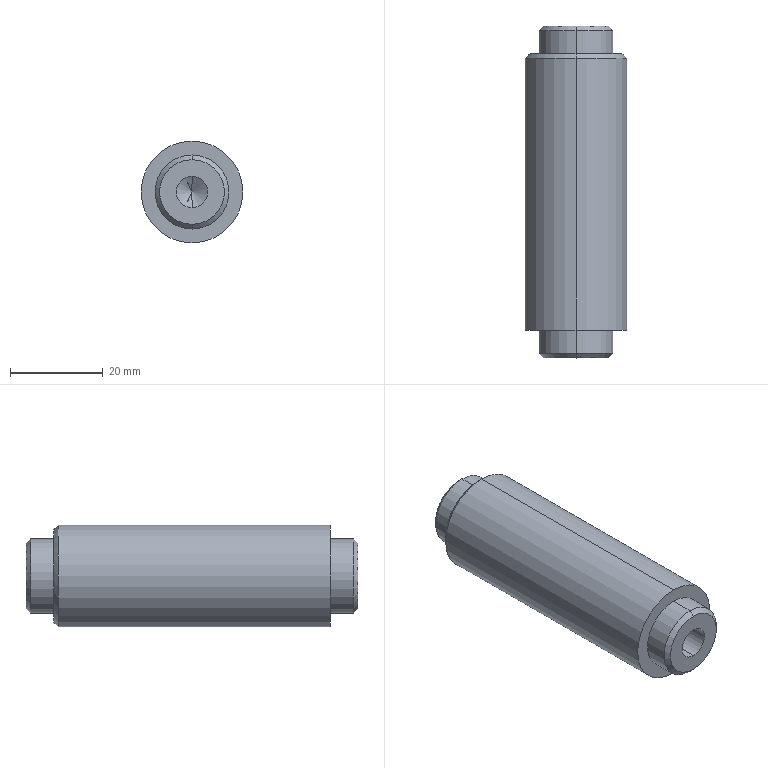Part | STEP file | circular post dia22-16-M8 | 1 solid | 24 faces | box 22 x 71.7 x 22 mm | volume 23541 mm3 | cone 10 | cylinder 10 | plane 4 | commonest cylinder face diameters 6.8 x4 16 x4 22 x2
STEP:
#1=CARTESIAN_POINT('',(0.,0.,0.));
#2=DIRECTION('',(0.,0.,1.));
#3=DIRECTION('',(1.,0.,0.));
#4=AXIS2_PLACEMENT_3D('',#1,#2,#3);
#5=CARTESIAN_POINT('',(0.,65.7,7.));
#6=VERTEX_POINT('',#5);
#7=CARTESIAN_POINT('',(0.,65.7,-7.));
#8=VERTEX_POINT('',#7);
#9=CARTESIAN_POINT('',(0.,65.7,0.));
#10=DIRECTION('',(0.,1.,0.));
#11=DIRECTION('',(0.,0.,1.));
#12=AXIS2_PLACEMENT_3D('',#9,#10,#11);
#13=CIRCLE('',#12,7.);
#14=CARTESIAN_POINT('',(0.,65.7,0.));
#15=DIRECTION('',(0.,-1.,0.));
#16=DIRECTION('',(0.,0.,-1.));
#17=AXIS2_PLACEMENT_3D('',#14,#15,#16);
#18=CONICAL_SURFACE('',#17,7.,0.7854);
#19=CARTESIAN_POINT('',(3.142,0.));
#20=DIRECTION('',(-1.,0.));
#21=VECTOR('',#20,1.);
#22=LINE('',#19,#21);
#23=(GEOMETRIC_REPRESENTATION_CONTEXT(2)PARAMETRIC_REPRESENTATION_CONTEXT()REPRESENTATION_CONTEXT('',''));
#24=DEFINITIONAL_REPRESENTATION('',(#22),#23);
#25=PCURVE('',#18,#24);
#26=CARTESIAN_POINT('',(0.,65.7,0.));
#27=DIRECTION('',(0.,1.,0.));
#28=DIRECTION('',(0.,0.,1.));
#29=AXIS2_PLACEMENT_3D('',#26,#27,#28);
#30=PLANE('',#29);
#31=CARTESIAN_POINT('',(0.,0.));
#32=DIRECTION('',(1.,0.));
#33=AXIS2_PLACEMENT_2D('',#31,#32);
#34=CIRCLE('',#33,7.);
#35=(GEOMETRIC_REPRESENTATION_CONTEXT(2)PARAMETRIC_REPRESENTATION_CONTEXT()REPRESENTATION_CONTEXT('',''));
#36=DEFINITIONAL_REPRESENTATION('',(#34),#35);
#37=PCURVE('',#30,#36);
#38=SURFACE_CURVE('',#13,(#25,#37),.PCURVE_S1.);
#39=EDGE_CURVE('',#6,#8,#38,.T.);
#40=ORIENTED_EDGE('',*,*,#39,.F.);
#41=CARTESIAN_POINT('',(0.,64.7,8.));
#42=VERTEX_POINT('',#41);
#43=CARTESIAN_POINT('',(0.,65.7,7.));
#44=DIRECTION('',(0.,-0.7071,0.7071));
#45=VECTOR('',#44,1.);
#46=LINE('',#43,#45);
#47=CARTESIAN_POINT('',(3.142,0.));
#48=DIRECTION('',(0.,1.));
#49=VECTOR('',#48,1.);
#50=LINE('',#47,#49);
#51=(GEOMETRIC_REPRESENTATION_CONTEXT(2)PARAMETRIC_REPRESENTATION_CONTEXT()REPRESENTATION_CONTEXT('',''));
#52=DEFINITIONAL_REPRESENTATION('',(#50),#51);
#53=PCURVE('',#18,#52);
#54=CARTESIAN_POINT('',(0.,65.7,0.));
#55=DIRECTION('',(0.,-1.,0.));
#56=DIRECTION('',(0.,0.,-1.));
#57=AXIS2_PLACEMENT_3D('',#54,#55,#56);
#58=CONICAL_SURFACE('',#57,7.,0.7854);
#59=CARTESIAN_POINT('',(3.142,0.));
#60=DIRECTION('',(0.,1.));
#61=VECTOR('',#60,1.);
#62=LINE('',#59,#61);
#63=(GEOMETRIC_REPRESENTATION_CONTEXT(2)PARAMETRIC_REPRESENTATION_CONTEXT()REPRESENTATION_CONTEXT('',''));
#64=DEFINITIONAL_REPRESENTATION('',(#62),#63);
#65=PCURVE('',#58,#64);
#66=SURFACE_CURVE('',#46,(#53,#65),.PCURVE_S1.);
#67=EDGE_CURVE('',#6,#42,#66,.T.);
#68=ORIENTED_EDGE('',*,*,#67,.T.);
#69=CARTESIAN_POINT('',(0.,64.7,-8.));
#70=VERTEX_POINT('',#69);
#71=CARTESIAN_POINT('',(0.,64.7,0.));
#72=DIRECTION('',(0.,-1.,0.));
#73=DIRECTION('',(0.,0.,1.));
#74=AXIS2_PLACEMENT_3D('',#71,#72,#73);
#75=CIRCLE('',#74,8.);
#76=CARTESIAN_POINT('',(-3.142,1.));
#77=DIRECTION('',(1.,0.));
#78=VECTOR('',#77,1.);
#79=LINE('',#76,#78);
#80=(GEOMETRIC_REPRESENTATION_CONTEXT(2)PARAMETRIC_REPRESENTATION_CONTEXT()REPRESENTATION_CONTEXT('',''));
#81=DEFINITIONAL_REPRESENTATION('',(#79),#80);
#82=PCURVE('',#18,#81);
#83=CARTESIAN_POINT('',(0.,65.7,0.));
#84=DIRECTION('',(0.,-1.,0.));
#85=DIRECTION('',(0.,0.,-1.));
#86=AXIS2_PLACEMENT_3D('',#83,#84,#85);
#87=CYLINDRICAL_SURFACE('',#86,8.);
#88=CARTESIAN_POINT('',(-3.142,1.));
#89=DIRECTION('',(1.,0.));
#90=VECTOR('',#89,1.);
#91=LINE('',#88,#90);
#92=(GEOMETRIC_REPRESENTATION_CONTEXT(2)PARAMETRIC_REPRESENTATION_CONTEXT()REPRESENTATION_CONTEXT('',''));
#93=DEFINITIONAL_REPRESENTATION('',(#91),#92);
#94=PCURVE('',#87,#93);
#95=SURFACE_CURVE('',#75,(#82,#94),.PCURVE_S1.);
#96=EDGE_CURVE('',#70,#42,#95,.T.);
#97=ORIENTED_EDGE('',*,*,#96,.F.);
#98=CARTESIAN_POINT('',(0.,65.7,-7.));
#99=DIRECTION('',(0.,-0.7071,-0.7071));
#100=VECTOR('',#99,1.);
#101=LINE('',#98,#100);
#102=CARTESIAN_POINT('',(0.,0.));
#103=DIRECTION('',(0.,1.));
#104=VECTOR('',#103,1.);
#105=LINE('',#102,#104);
#106=(GEOMETRIC_REPRESENTATION_CONTEXT(2)PARAMETRIC_REPRESENTATION_CONTEXT()REPRESENTATION_CONTEXT('',''));
#107=DEFINITIONAL_REPRESENTATION('',(#105),#106);
#108=PCURVE('',#18,#107);
#109=CARTESIAN_POINT('',(6.283,0.));
#110=DIRECTION('',(0.,1.));
#111=VECTOR('',#110,1.);
#112=LINE('',#109,#111);
#113=(GEOMETRIC_REPRESENTATION_CONTEXT(2)PARAMETRIC_REPRESENTATION_CONTEXT()REPRESENTATION_CONTEXT('',''));
#114=DEFINITIONAL_REPRESENTATION('',(#112),#113);
#115=PCURVE('',#58,#114);
#116=SURFACE_CURVE('',#101,(#108,#115),.PCURVE_S1.);
#117=EDGE_CURVE('',#8,#70,#116,.T.);
#118=ORIENTED_EDGE('',*,*,#117,.F.);
#119=EDGE_LOOP('',(#40,#68,#97,#118));
#120=FACE_BOUND('',#119,.T.);
#121=ADVANCED_FACE('',(#120),#18,.T.);
#122=CARTESIAN_POINT('',(0.,45.95,3.4));
#123=VERTEX_POINT('',#122);
#124=CARTESIAN_POINT('',(0.,65.7,3.4));
#125=VERTEX_POINT('',#124);
#126=CARTESIAN_POINT('',(0.,65.7,3.4));
#127=DIRECTION('',(0.,1.,0.));
#128=VECTOR('',#127,1.);
#129=LINE('',#126,#128);
#130=CARTESIAN_POINT('',(0.,65.7,0.));
#131=DIRECTION('',(0.,1.,0.));
#132=DIRECTION('',(0.,0.,1.));
#133=AXIS2_PLACEMENT_3D('',#130,#131,#132);
#134=CYLINDRICAL_SURFACE('',#133,3.4);
#135=CARTESIAN_POINT('',(6.283,0.));
#136=DIRECTION('',(0.,1.));
#137=VECTOR('',#136,1.);
#138=LINE('',#135,#137);
#139=(GEOMETRIC_REPRESENTATION_CONTEXT(2)PARAMETRIC_REPRESENTATION_CONTEXT()REPRESENTATION_CONTEXT('',''));
#140=DEFINITIONAL_REPRESENTATION('',(#138),#139);
#141=PCURVE('',#134,#140);
#142=CARTESIAN_POINT('',(0.,65.7,0.));
#143=DIRECTION('',(0.,1.,0.));
#144=DIRECTION('',(0.,0.,1.));
#145=AXIS2_PLACEMENT_3D('',#142,#143,#144);
#146=CYLINDRICAL_SURFACE('',#145,3.4);
#147=CARTESIAN_POINT('',(0.,0.));
#148=DIRECTION('',(0.,1.));
#149=VECTOR('',#148,1.);
#150=LINE('',#147,#149);
#151=(GEOMETRIC_REPRESENTATION_CONTEXT(2)PARAMETRIC_REPRESENTATION_CONTEXT()REPRESENTATION_CONTEXT('',''));
#152=DEFINITIONAL_REPRESENTATION('',(#150),#151);
#153=PCURVE('',#146,#152);
#154=SURFACE_CURVE('',#129,(#141,#153),.PCURVE_S1.);
#155=EDGE_CURVE('',#123,#125,#154,.T.);
#156=ORIENTED_EDGE('',*,*,#155,.T.);
#157=CARTESIAN_POINT('',(0.,65.7,-3.4));
#158=VERTEX_POINT('',#157);
#159=CARTESIAN_POINT('',(0.,65.7,0.));
#160=DIRECTION('',(0.,1.,0.));
#161=DIRECTION('',(0.,0.,1.));
#162=AXIS2_PLACEMENT_3D('',#159,#160,#161);
#163=CIRCLE('',#162,3.4);
#164=CARTESIAN_POINT('',(0.,0.));
#165=DIRECTION('',(1.,0.));
#166=VECTOR('',#165,1.);
#167=LINE('',#164,#166);
#168=(GEOMETRIC_REPRESENTATION_CONTEXT(2)PARAMETRIC_REPRESENTATION_CONTEXT()REPRESENTATION_CONTEXT('',''));
#169=DEFINITIONAL_REPRESENTATION('',(#167),#168);
#170=PCURVE('',#134,#169);
#171=CARTESIAN_POINT('',(0.,0.));
#172=DIRECTION('',(1.,0.));
#173=AXIS2_PLACEMENT_2D('',#171,#172);
#174=CIRCLE('',#173,3.4);
#175=(GEOMETRIC_REPRESENTATION_CONTEXT(2)PARAMETRIC_REPRESENTATION_CONTEXT()REPRESENTATION_CONTEXT('',''));
#176=DEFINITIONAL_REPRESENTATION('',(#174),#175);
#177=PCURVE('',#30,#176);
#178=SURFACE_CURVE('',#163,(#170,#177),.PCURVE_S1.);
#179=EDGE_CURVE('',#158,#125,#178,.T.);
#180=ORIENTED_EDGE('',*,*,#179,.F.);
#181=CARTESIAN_POINT('',(0.,45.95,-3.4));
#182=VERTEX_POINT('',#181);
#183=CARTESIAN_POINT('',(0.,65.7,-3.4));
#184=DIRECTION('',(0.,1.,0.));
#185=VECTOR('',#184,1.);
#186=LINE('',#183,#185);
#187=CARTESIAN_POINT('',(3.142,0.));
#188=DIRECTION('',(0.,1.));
#189=VECTOR('',#188,1.);
#190=LINE('',#187,#189);
#191=(GEOMETRIC_REPRESENTATION_CONTEXT(2)PARAMETRIC_REPRESENTATION_CONTEXT()REPRESENTATION_CONTEXT('',''));
#192=DEFINITIONAL_REPRESENTATION('',(#190),#191);
#193=PCURVE('',#134,#192);
#194=CARTESIAN_POINT('',(3.142,0.));
#195=DIRECTION('',(0.,1.));
#196=VECTOR('',#195,1.);
#197=LINE('',#194,#196);
#198=(GEOMETRIC_REPRESENTATION_CONTEXT(2)PARAMETRIC_REPRESENTATION_CONTEXT()REPRESENTATION_CONTEXT('',''));
#199=DEFINITIONAL_REPRESENTATION('',(#197),#198);
#200=PCURVE('',#146,#199);
#201=SURFACE_CURVE('',#186,(#193,#200),.PCURVE_S1.);
#202=EDGE_CURVE('',#182,#158,#201,.T.);
#203=ORIENTED_EDGE('',*,*,#202,.F.);
#204=CARTESIAN_POINT('',(0.,45.95,0.));
#205=DIRECTION('',(0.,1.,0.));
#206=DIRECTION('',(0.,0.,1.));
#207=AXIS2_PLACEMENT_3D('',#204,#205,#206);
#208=CIRCLE('',#207,3.4);
#209=CARTESIAN_POINT('',(0.,-19.75));
#210=DIRECTION('',(1.,0.));
#211=VECTOR('',#210,1.);
#212=LINE('',#209,#211);
#213=(GEOMETRIC_REPRESENTATION_CONTEXT(2)PARAMETRIC_REPRESENTATION_CONTEXT()REPRESENTATION_CONTEXT('',''));
#214=DEFINITIONAL_REPRESENTATION('',(#212),#213);
#215=PCURVE('',#134,#214);
#216=CARTESIAN_POINT('',(0.,45.95,0.));
#217=DIRECTION('',(0.,1.,0.));
#218=DIRECTION('',(0.,0.,1.));
#219=AXIS2_PLACEMENT_3D('',#216,#217,#218);
#220=CONICAL_SURFACE('',#219,3.4,1.03);
#221=CARTESIAN_POINT('',(0.,0.));
#222=DIRECTION('',(1.,0.));
#223=VECTOR('',#222,1.);
#224=LINE('',#221,#223);
#225=(GEOMETRIC_REPRESENTATION_CONTEXT(2)PARAMETRIC_REPRESENTATION_CONTEXT()REPRESENTATION_CONTEXT('',''));
#226=DEFINITIONAL_REPRESENTATION('',(#224),#225);
#227=PCURVE('',#220,#226);
#228=SURFACE_CURVE('',#208,(#215,#227),.PCURVE_S1.);
#229=EDGE_CURVE('',#182,#123,#228,.T.);
#230=ORIENTED_EDGE('',*,*,#229,.T.);
#231=EDGE_LOOP('',(#156,#180,#203,#230));
#232=FACE_BOUND('',#231,.F.);
#233=ADVANCED_FACE('',(#232),#134,.F.);
#234=ORIENTED_EDGE('',*,*,#229,.F.);
#235=CARTESIAN_POINT('',(0.,43.907,0.));
#236=VERTEX_POINT('',#235);
#237=CARTESIAN_POINT('',(0.,45.95,-3.4));
#238=DIRECTION('',(0.,0.515,-0.8572));
#239=VECTOR('',#238,1.);
#240=LINE('',#237,#239);
#241=CARTESIAN_POINT('',(3.142,0.));
#242=DIRECTION('',(0.,1.));
#243=VECTOR('',#242,1.);
#244=LINE('',#241,#243);
#245=(GEOMETRIC_REPRESENTATION_CONTEXT(2)PARAMETRIC_REPRESENTATION_CONTEXT()REPRESENTATION_CONTEXT('',''));
#246=DEFINITIONAL_REPRESENTATION('',(#244),#245);
#247=PCURVE('',#220,#246);
#248=CARTESIAN_POINT('',(0.,45.95,0.));
#249=DIRECTION('',(0.,1.,0.));
#250=DIRECTION('',(0.,0.,1.));
#251=AXIS2_PLACEMENT_3D('',#248,#249,#250);
#252=CONICAL_SURFACE('',#251,3.4,1.03);
#253=CARTESIAN_POINT('',(3.142,0.));
#254=DIRECTION('',(0.,1.));
#255=VECTOR('',#254,1.);
#256=LINE('',#253,#255);
#257=(GEOMETRIC_REPRESENTATION_CONTEXT(2)PARAMETRIC_REPRESENTATION_CONTEXT()REPRESENTATION_CONTEXT('',''));
#258=DEFINITIONAL_REPRESENTATION('',(#256),#257);
#259=PCURVE('',#252,#258);
#260=SURFACE_CURVE('',#240,(#247,#259),.PCURVE_S1.);
#261=EDGE_CURVE('',#236,#182,#260,.T.);
#262=ORIENTED_EDGE('',*,*,#261,.F.);
#263=CARTESIAN_POINT('',(0.,45.95,3.4));
#264=DIRECTION('',(0.,0.515,0.8572));
#265=VECTOR('',#264,1.);
#266=LINE('',#263,#265);
#267=CARTESIAN_POINT('',(6.283,0.));
#268=DIRECTION('',(0.,1.));
#269=VECTOR('',#268,1.);
#270=LINE('',#267,#269);
#271=(GEOMETRIC_REPRESENTATION_CONTEXT(2)PARAMETRIC_REPRESENTATION_CONTEXT()REPRESENTATION_CONTEXT('',''));
#272=DEFINITIONAL_REPRESENTATION('',(#270),#271);
#273=PCURVE('',#220,#272);
#274=CARTESIAN_POINT('',(0.,0.));
#275=DIRECTION('',(0.,1.));
#276=VECTOR('',#275,1.);
#277=LINE('',#274,#276);
#278=(GEOMETRIC_REPRESENTATION_CONTEXT(2)PARAMETRIC_REPRESENTATION_CONTEXT()REPRESENTATION_CONTEXT('',''));
#279=DEFINITIONAL_REPRESENTATION('',(#277),#278);
#280=PCURVE('',#252,#279);
#281=SURFACE_CURVE('',#266,(#273,#280),.PCURVE_S1.);
#282=EDGE_CURVE('',#236,#123,#281,.T.);
#283=ORIENTED_EDGE('',*,*,#282,.T.);
#284=EDGE_LOOP('',(#234,#262,#283));
#285=FACE_BOUND('',#284,.F.);
#286=ADVANCED_FACE('',(#285),#220,.F.);
#287=ORIENTED_EDGE('',*,*,#96,.T.);
#288=CARTESIAN_POINT('',(0.,59.7,8.));
#289=VERTEX_POINT('',#288);
#290=CARTESIAN_POINT('',(0.,65.7,8.));
#291=DIRECTION('',(0.,-1.,0.));
#292=VECTOR('',#291,1.);
#293=LINE('',#290,#292);
#294=CARTESIAN_POINT('',(3.142,0.));
#295=DIRECTION('',(0.,1.));
#296=VECTOR('',#295,1.);
#297=LINE('',#294,#296);
#298=(GEOMETRIC_REPRESENTATION_CONTEXT(2)PARAMETRIC_REPRESENTATION_CONTEXT()REPRESENTATION_CONTEXT('',''));
#299=DEFINITIONAL_REPRESENTATION('',(#297),#298);
#300=PCURVE('',#87,#299);
#301=CARTESIAN_POINT('',(0.,65.7,0.));
#302=DIRECTION('',(0.,-1.,0.));
#303=DIRECTION('',(0.,0.,-1.));
#304=AXIS2_PLACEMENT_3D('',#301,#302,#303);
#305=CYLINDRICAL_SURFACE('',#304,8.);
#306=CARTESIAN_POINT('',(3.142,0.));
#307=DIRECTION('',(0.,1.));
#308=VECTOR('',#307,1.);
#309=LINE('',#306,#308);
#310=(GEOMETRIC_REPRESENTATION_CONTEXT(2)PARAMETRIC_REPRESENTATION_CONTEXT()REPRESENTATION_CONTEXT('',''));
#311=DEFINITIONAL_REPRESENTATION('',(#309),#310);
#312=PCURVE('',#305,#311);
#313=SURFACE_CURVE('',#293,(#300,#312),.PCURVE_S1.);
#314=EDGE_CURVE('',#42,#289,#313,.T.);
#315=ORIENTED_EDGE('',*,*,#314,.T.);
#316=CARTESIAN_POINT('',(0.,59.7,-8.));
#317=VERTEX_POINT('',#316);
#318=CARTESIAN_POINT('',(0.,59.7,0.));
#319=DIRECTION('',(0.,1.,0.));
#320=DIRECTION('',(0.,0.,1.));
#321=AXIS2_PLACEMENT_3D('',#318,#319,#320);
#322=CIRCLE('',#321,8.);
#323=CARTESIAN_POINT('',(3.142,6.));
#324=DIRECTION('',(-1.,0.));
#325=VECTOR('',#324,1.);
#326=LINE('',#323,#325);
#327=(GEOMETRIC_REPRESENTATION_CONTEXT(2)PARAMETRIC_REPRESENTATION_CONTEXT()REPRESENTATION_CONTEXT('',''));
#328=DEFINITIONAL_REPRESENTATION('',(#326),#327);
#329=PCURVE('',#87,#328);
#330=CARTESIAN_POINT('',(0.,59.7,0.));
#331=DIRECTION('',(0.,1.,0.));
#332=DIRECTION('',(0.,0.,1.));
#333=AXIS2_PLACEMENT_3D('',#330,#331,#332);
#334=PLANE('',#333);
#335=CARTESIAN_POINT('',(0.,0.));
#336=DIRECTION('',(1.,0.));
#337=AXIS2_PLACEMENT_2D('',#335,#336);
#338=CIRCLE('',#337,8.);
#339=(GEOMETRIC_REPRESENTATION_CONTEXT(2)PARAMETRIC_REPRESENTATION_CONTEXT()REPRESENTATION_CONTEXT('',''));
#340=DEFINITIONAL_REPRESENTATION('',(#338),#339);
#341=PCURVE('',#334,#340);
#342=SURFACE_CURVE('',#322,(#329,#341),.PCURVE_S1.);
#343=EDGE_CURVE('',#289,#317,#342,.T.);
#344=ORIENTED_EDGE('',*,*,#343,.T.);
#345=CARTESIAN_POINT('',(0.,65.7,-8.));
#346=DIRECTION('',(0.,-1.,0.));
#347=VECTOR('',#346,1.);
#348=LINE('',#345,#347);
#349=CARTESIAN_POINT('',(0.,0.));
#350=DIRECTION('',(0.,1.));
#351=VECTOR('',#350,1.);
#352=LINE('',#349,#351);
#353=(GEOMETRIC_REPRESENTATION_CONTEXT(2)PARAMETRIC_REPRESENTATION_CONTEXT()REPRESENTATION_CONTEXT('',''));
#354=DEFINITIONAL_REPRESENTATION('',(#352),#353);
#355=PCURVE('',#87,#354);
#356=CARTESIAN_POINT('',(6.283,0.));
#357=DIRECTION('',(0.,1.));
#358=VECTOR('',#357,1.);
#359=LINE('',#356,#358);
#360=(GEOMETRIC_REPRESENTATION_CONTEXT(2)PARAMETRIC_REPRESENTATION_CONTEXT()REPRESENTATION_CONTEXT('',''));
#361=DEFINITIONAL_REPRESENTATION('',(#359),#360);
#362=PCURVE('',#305,#361);
#363=SURFACE_CURVE('',#348,(#355,#362),.PCURVE_S1.);
#364=EDGE_CURVE('',#70,#317,#363,.T.);
#365=ORIENTED_EDGE('',*,*,#364,.F.);
#366=EDGE_LOOP('',(#287,#315,#344,#365));
#367=FACE_BOUND('',#366,.T.);
#368=ADVANCED_FACE('',(#367),#87,.T.);
#369=CARTESIAN_POINT('',(0.,59.7,10.));
#370=VERTEX_POINT('',#369);
#371=CARTESIAN_POINT('',(0.,59.7,-10.));
#372=VERTEX_POINT('',#371);
#373=CARTESIAN_POINT('',(0.,59.7,0.));
#374=DIRECTION('',(0.,1.,0.));
#375=DIRECTION('',(0.,0.,1.));
#376=AXIS2_PLACEMENT_3D('',#373,#374,#375);
#377=CIRCLE('',#376,10.);
#378=CARTESIAN_POINT('',(0.,59.7,0.));
#379=DIRECTION('',(0.,-1.,0.));
#380=DIRECTION('',(0.,0.,-1.));
#381=AXIS2_PLACEMENT_3D('',#378,#379,#380);
#382=CONICAL_SURFACE('',#381,10.,0.7854);
#383=CARTESIAN_POINT('',(3.142,0.));
#384=DIRECTION('',(-1.,0.));
#385=VECTOR('',#384,1.);
#386=LINE('',#383,#385);
#387=(GEOMETRIC_REPRESENTATION_CONTEXT(2)PARAMETRIC_REPRESENTATION_CONTEXT()REPRESENTATION_CONTEXT('',''));
#388=DEFINITIONAL_REPRESENTATION('',(#386),#387);
#389=PCURVE('',#382,#388);
#390=CARTESIAN_POINT('',(0.,0.));
#391=DIRECTION('',(1.,0.));
#392=AXIS2_PLACEMENT_2D('',#390,#391);
#393=CIRCLE('',#392,10.);
#394=(GEOMETRIC_REPRESENTATION_CONTEXT(2)PARAMETRIC_REPRESENTATION_CONTEXT()REPRESENTATION_CONTEXT('',''));
#395=DEFINITIONAL_REPRESENTATION('',(#393),#394);
#396=PCURVE('',#334,#395);
#397=SURFACE_CURVE('',#377,(#389,#396),.PCURVE_S1.);
#398=EDGE_CURVE('',#370,#372,#397,.T.);
#399=ORIENTED_EDGE('',*,*,#398,.F.);
#400=CARTESIAN_POINT('',(0.,58.7,11.));
#401=VERTEX_POINT('',#400);
#402=CARTESIAN_POINT('',(0.,59.7,10.));
#403=DIRECTION('',(0.,-0.7071,0.7071));
#404=VECTOR('',#403,1.);
#405=LINE('',#402,#404);
#406=CARTESIAN_POINT('',(3.142,0.));
#407=DIRECTION('',(0.,1.));
#408=VECTOR('',#407,1.);
#409=LINE('',#406,#408);
#410=(GEOMETRIC_REPRESENTATION_CONTEXT(2)PARAMETRIC_REPRESENTATION_CONTEXT()REPRESENTATION_CONTEXT('',''));
#411=DEFINITIONAL_REPRESENTATION('',(#409),#410);
#412=PCURVE('',#382,#411);
#413=CARTESIAN_POINT('',(0.,59.7,0.));
#414=DIRECTION('',(0.,-1.,0.));
#415=DIRECTION('',(0.,0.,-1.));
#416=AXIS2_PLACEMENT_3D('',#413,#414,#415);
#417=CONICAL_SURFACE('',#416,10.,0.7854);
#418=CARTESIAN_POINT('',(3.142,0.));
#419=DIRECTION('',(0.,1.));
#420=VECTOR('',#419,1.);
#421=LINE('',#418,#420);
#422=(GEOMETRIC_REPRESENTATION_CONTEXT(2)PARAMETRIC_REPRESENTATION_CONTEXT()REPRESENTATION_CONTEXT('',''));
#423=DEFINITIONAL_REPRESENTATION('',(#421),#422);
#424=PCURVE('',#417,#423);
#425=SURFACE_CURVE('',#405,(#412,#424),.PCURVE_S1.);
#426=EDGE_CURVE('',#370,#401,#425,.T.);
#427=ORIENTED_EDGE('',*,*,#426,.T.);
#428=CARTESIAN_POINT('',(0.,58.7,-11.));
#429=VERTEX_POINT('',#428);
#430=CARTESIAN_POINT('',(0.,58.7,0.));
#431=DIRECTION('',(0.,-1.,0.));
#432=DIRECTION('',(0.,0.,1.));
#433=AXIS2_PLACEMENT_3D('',#430,#431,#432);
#434=CIRCLE('',#433,11.);
#435=CARTESIAN_POINT('',(-3.142,1.));
#436=DIRECTION('',(1.,0.));
#437=VECTOR('',#436,1.);
#438=LINE('',#435,#437);
#439=(GEOMETRIC_REPRESENTATION_CONTEXT(2)PARAMETRIC_REPRESENTATION_CONTEXT()REPRESENTATION_CONTEXT('',''));
#440=DEFINITIONAL_REPRESENTATION('',(#438),#439);
#441=PCURVE('',#382,#440);
#442=CARTESIAN_POINT('',(0.,59.7,0.));
#443=DIRECTION('',(0.,-1.,0.));
#444=DIRECTION('',(0.,0.,-1.));
#445=AXIS2_PLACEMENT_3D('',#442,#443,#444);
#446=CYLINDRICAL_SURFACE('',#445,11.);
#447=CARTESIAN_POINT('',(-3.142,1.));
#448=DIRECTION('',(1.,0.));
#449=VECTOR('',#448,1.);
#450=LINE('',#447,#449);
#451=(GEOMETRIC_REPRESENTATION_CONTEXT(2)PARAMETRIC_REPRESENTATION_CONTEXT()REPRESENTATION_CONTEXT('',''));
#452=DEFINITIONAL_REPRESENTATION('',(#450),#451);
#453=PCURVE('',#446,#452);
#454=SURFACE_CURVE('',#434,(#441,#453),.PCURVE_S1.);
#455=EDGE_CURVE('',#429,#401,#454,.T.);
#456=ORIENTED_EDGE('',*,*,#455,.F.);
#457=CARTESIAN_POINT('',(0.,59.7,-10.));
#458=DIRECTION('',(0.,-0.7071,-0.7071));
#459=VECTOR('',#458,1.);
#460=LINE('',#457,#459);
#461=CARTESIAN_POINT('',(0.,0.));
#462=DIRECTION('',(0.,1.));
#463=VECTOR('',#462,1.);
#464=LINE('',#461,#463);
#465=(GEOMETRIC_REPRESENTATION_CONTEXT(2)PARAMETRIC_REPRESENTATION_CONTEXT()REPRESENTATION_CONTEXT('',''));
#466=DEFINITIONAL_REPRESENTATION('',(#464),#465);
#467=PCURVE('',#382,#466);
#468=CARTESIAN_POINT('',(6.283,0.));
#469=DIRECTION('',(0.,1.));
#470=VECTOR('',#469,1.);
#471=LINE('',#468,#470);
#472=(GEOMETRIC_REPRESENTATION_CONTEXT(2)PARAMETRIC_REPRESENTATION_CONTEXT()REPRESENTATION_CONTEXT('',''));
#473=DEFINITIONAL_REPRESENTATION('',(#471),#472);
#474=PCURVE('',#417,#473);
#475=SURFACE_CURVE('',#460,(#467,#474),.PCURVE_S1.);
#476=EDGE_CURVE('',#372,#429,#475,.T.);
#477=ORIENTED_EDGE('',*,*,#476,.F.);
#478=EDGE_LOOP('',(#399,#427,#456,#477));
#479=FACE_BOUND('',#478,.T.);
#480=ADVANCED_FACE('',(#479),#382,.T.);
#481=CARTESIAN_POINT('',(0.,13.75,-3.4));
#482=VERTEX_POINT('',#481);
#483=CARTESIAN_POINT('',(0.,-6.,-3.4));
#484=VERTEX_POINT('',#483);
#485=CARTESIAN_POINT('',(0.,-6.,-3.4));
#486=DIRECTION('',(0.,-1.,0.));
#487=VECTOR('',#486,1.);
#488=LINE('',#485,#487);
#489=CARTESIAN_POINT('',(0.,-6.,0.));
#490=DIRECTION('',(0.,-1.,0.));
#491=DIRECTION('',(0.,0.,-1.));
#492=AXIS2_PLACEMENT_3D('',#489,#490,#491);
#493=CYLINDRICAL_SURFACE('',#492,3.4);
#494=CARTESIAN_POINT('',(6.283,0.));
#495=DIRECTION('',(0.,1.));
#496=VECTOR('',#495,1.);
#497=LINE('',#494,#496);
#498=(GEOMETRIC_REPRESENTATION_CONTEXT(2)PARAMETRIC_REPRESENTATION_CONTEXT()REPRESENTATION_CONTEXT('',''));
#499=DEFINITIONAL_REPRESENTATION('',(#497),#498);
#500=PCURVE('',#493,#499);
#501=CARTESIAN_POINT('',(0.,-6.,0.));
#502=DIRECTION('',(0.,-1.,0.));
#503=DIRECTION('',(0.,0.,-1.));
#504=AXIS2_PLACEMENT_3D('',#501,#502,#503);
#505=CYLINDRICAL_SURFACE('',#504,3.4);
#506=CARTESIAN_POINT('',(0.,0.));
#507=DIRECTION('',(0.,1.));
#508=VECTOR('',#507,1.);
#509=LINE('',#506,#508);
#510=(GEOMETRIC_REPRESENTATION_CONTEXT(2)PARAMETRIC_REPRESENTATION_CONTEXT()REPRESENTATION_CONTEXT('',''));
#511=DEFINITIONAL_REPRESENTATION('',(#509),#510);
#512=PCURVE('',#505,#511);
#513=SURFACE_CURVE('',#488,(#500,#512),.PCURVE_S1.);
#514=EDGE_CURVE('',#482,#484,#513,.T.);
#515=ORIENTED_EDGE('',*,*,#514,.T.);
#516=CARTESIAN_POINT('',(0.,-6.,3.4));
#517=VERTEX_POINT('',#516);
#518=CARTESIAN_POINT('',(0.,-6.,0.));
#519=DIRECTION('',(0.,-1.,0.));
#520=DIRECTION('',(0.,0.,-1.));
#521=AXIS2_PLACEMENT_3D('',#518,#519,#520);
#522=CIRCLE('',#521,3.4);
#523=CARTESIAN_POINT('',(0.,0.));
#524=DIRECTION('',(1.,0.));
#525=VECTOR('',#524,1.);
#526=LINE('',#523,#525);
#527=(GEOMETRIC_REPRESENTATION_CONTEXT(2)PARAMETRIC_REPRESENTATION_CONTEXT()REPRESENTATION_CONTEXT('',''));
#528=DEFINITIONAL_REPRESENTATION('',(#526),#527);
#529=PCURVE('',#493,#528);
#530=CARTESIAN_POINT('',(0.,-6.,0.));
#531=DIRECTION('',(0.,-1.,0.));
#532=DIRECTION('',(0.,0.,-1.));
#533=AXIS2_PLACEMENT_3D('',#530,#531,#532);
#534=PLANE('',#533);
#535=CARTESIAN_POINT('',(0.,0.));
#536=DIRECTION('',(1.,0.));
#537=AXIS2_PLACEMENT_2D('',#535,#536);
#538=CIRCLE('',#537,3.4);
#539=(GEOMETRIC_REPRESENTATION_CONTEXT(2)PARAMETRIC_REPRESENTATION_CONTEXT()REPRESENTATION_CONTEXT('',''));
#540=DEFINITIONAL_REPRESENTATION('',(#538),#539);
#541=PCURVE('',#534,#540);
#542=SURFACE_CURVE('',#522,(#529,#541),.PCURVE_S1.);
#543=EDGE_CURVE('',#517,#484,#542,.T.);
#544=ORIENTED_EDGE('',*,*,#543,.F.);
#545=CARTESIAN_POINT('',(0.,13.75,3.4));
#546=VERTEX_POINT('',#545);
#547=CARTESIAN_POINT('',(0.,-6.,3.4));
#548=DIRECTION('',(0.,-1.,0.));
#549=VECTOR('',#548,1.);
#550=LINE('',#547,#549);
#551=CARTESIAN_POINT('',(3.142,0.));
#552=DIRECTION('',(0.,1.));
#553=VECTOR('',#552,1.);
#554=LINE('',#551,#553);
#555=(GEOMETRIC_REPRESENTATION_CONTEXT(2)PARAMETRIC_REPRESENTATION_CONTEXT()REPRESENTATION_CONTEXT('',''));
#556=DEFINITIONAL_REPRESENTATION('',(#554),#555);
#557=PCURVE('',#493,#556);
#558=CARTESIAN_POINT('',(3.142,0.));
#559=DIRECTION('',(0.,1.));
#560=VECTOR('',#559,1.);
#561=LINE('',#558,#560);
#562=(GEOMETRIC_REPRESENTATION_CONTEXT(2)PARAMETRIC_REPRESENTATION_CONTEXT()REPRESENTATION_CONTEXT('',''));
#563=DEFINITIONAL_REPRESENTATION('',(#561),#562);
#564=PCURVE('',#505,#563);
#565=SURFACE_CURVE('',#550,(#557,#564),.PCURVE_S1.);
#566=EDGE_CURVE('',#546,#517,#565,.T.);
#567=ORIENTED_EDGE('',*,*,#566,.F.);
#568=CARTESIAN_POINT('',(0.,13.75,0.));
#569=DIRECTION('',(0.,-1.,0.));
#570=DIRECTION('',(0.,0.,-1.));
#571=AXIS2_PLACEMENT_3D('',#568,#569,#570);
#572=CIRCLE('',#571,3.4);
#573=CARTESIAN_POINT('',(0.,-19.75));
#574=DIRECTION('',(1.,0.));
#575=VECTOR('',#574,1.);
#576=LINE('',#573,#575);
#577=(GEOMETRIC_REPRESENTATION_CONTEXT(2)PARAMETRIC_REPRESENTATION_CONTEXT()REPRESENTATION_CONTEXT('',''));
#578=DEFINITIONAL_REPRESENTATION('',(#576),#577);
#579=PCURVE('',#493,#578);
#580=CARTESIAN_POINT('',(0.,13.75,0.));
#581=DIRECTION('',(0.,-1.,0.));
#582=DIRECTION('',(0.,0.,-1.));
#583=AXIS2_PLACEMENT_3D('',#580,#581,#582);
#584=CONICAL_SURFACE('',#583,3.4,1.03);
#585=CARTESIAN_POINT('',(0.,0.));
#586=DIRECTION('',(1.,0.));
#587=VECTOR('',#586,1.);
#588=LINE('',#585,#587);
#589=(GEOMETRIC_REPRESENTATION_CONTEXT(2)PARAMETRIC_REPRESENTATION_CONTEXT()REPRESENTATION_CONTEXT('',''));
#590=DEFINITIONAL_REPRESENTATION('',(#588),#589);
#591=PCURVE('',#584,#590);
#592=SURFACE_CURVE('',#572,(#579,#591),.PCURVE_S1.);
#593=EDGE_CURVE('',#546,#482,#592,.T.);
#594=ORIENTED_EDGE('',*,*,#593,.T.);
#595=EDGE_LOOP('',(#515,#544,#567,#594));
#596=FACE_BOUND('',#595,.F.);
#597=ADVANCED_FACE('',(#596),#493,.F.);
#598=ORIENTED_EDGE('',*,*,#593,.F.);
#599=CARTESIAN_POINT('',(0.,15.793,0.));
#600=VERTEX_POINT('',#599);
#601=CARTESIAN_POINT('',(0.,13.75,3.4));
#602=DIRECTION('',(0.,-0.515,0.8572));
#603=VECTOR('',#602,1.);
#604=LINE('',#601,#603);
#605=CARTESIAN_POINT('',(3.142,0.));
#606=DIRECTION('',(0.,1.));
#607=VECTOR('',#606,1.);
#608=LINE('',#605,#607);
#609=(GEOMETRIC_REPRESENTATION_CONTEXT(2)PARAMETRIC_REPRESENTATION_CONTEXT()REPRESENTATION_CONTEXT('',''));
#610=DEFINITIONAL_REPRESENTATION('',(#608),#609);
#611=PCURVE('',#584,#610);
#612=CARTESIAN_POINT('',(0.,13.75,0.));
#613=DIRECTION('',(0.,-1.,0.));
#614=DIRECTION('',(0.,0.,-1.));
#615=AXIS2_PLACEMENT_3D('',#612,#613,#614);
#616=CONICAL_SURFACE('',#615,3.4,1.03);
#617=CARTESIAN_POINT('',(3.142,0.));
#618=DIRECTION('',(0.,1.));
#619=VECTOR('',#618,1.);
#620=LINE('',#617,#619);
#621=(GEOMETRIC_REPRESENTATION_CONTEXT(2)PARAMETRIC_REPRESENTATION_CONTEXT()REPRESENTATION_CONTEXT('',''));
#622=DEFINITIONAL_REPRESENTATION('',(#620),#621);
#623=PCURVE('',#616,#622);
#624=SURFACE_CURVE('',#604,(#611,#623),.PCURVE_S1.);
#625=EDGE_CURVE('',#600,#546,#624,.T.);
#626=ORIENTED_EDGE('',*,*,#625,.F.);
#627=CARTESIAN_POINT('',(0.,13.75,-3.4));
#628=DIRECTION('',(0.,-0.515,-0.8572));
#629=VECTOR('',#628,1.);
#630=LINE('',#627,#629);
#631=CARTESIAN_POINT('',(6.283,0.));
#632=DIRECTION('',(0.,1.));
#633=VECTOR('',#632,1.);
#634=LINE('',#631,#633);
#635=(GEOMETRIC_REPRESENTATION_CONTEXT(2)PARAMETRIC_REPRESENTATION_CONTEXT()REPRESENTATION_CONTEXT('',''));
#636=DEFINITIONAL_REPRESENTATION('',(#634),#635);
#637=PCURVE('',#584,#636);
#638=CARTESIAN_POINT('',(0.,0.));
#639=DIRECTION('',(0.,1.));
#640=VECTOR('',#639,1.);
#641=LINE('',#638,#640);
#642=(GEOMETRIC_REPRESENTATION_CONTEXT(2)PARAMETRIC_REPRESENTATION_CONTEXT()REPRESENTATION_CONTEXT('',''));
#643=DEFINITIONAL_REPRESENTATION('',(#641),#642);
#644=PCURVE('',#616,#643);
#645=SURFACE_CURVE('',#630,(#637,#644),.PCURVE_S1.);
#646=EDGE_CURVE('',#600,#482,#645,.T.);
#647=ORIENTED_EDGE('',*,*,#646,.T.);
#648=EDGE_LOOP('',(#598,#626,#647));
#649=FACE_BOUND('',#648,.F.);
#650=ADVANCED_FACE('',(#649),#584,.F.);
#651=CARTESIAN_POINT('',(0.,-6.,-7.));
#652=VERTEX_POINT('',#651);
#653=CARTESIAN_POINT('',(0.,-6.,7.));
#654=VERTEX_POINT('',#653);
#655=CARTESIAN_POINT('',(0.,-6.,0.));
#656=DIRECTION('',(0.,-1.,0.));
#657=DIRECTION('',(0.,0.,-1.));
#658=AXIS2_PLACEMENT_3D('',#655,#656,#657);
#659=CIRCLE('',#658,7.);
#660=CARTESIAN_POINT('',(0.,-6.,0.));
#661=DIRECTION('',(0.,1.,0.));
#662=DIRECTION('',(0.,0.,1.));
#663=AXIS2_PLACEMENT_3D('',#660,#661,#662);
#664=CONICAL_SURFACE('',#663,7.,0.7854);
#665=CARTESIAN_POINT('',(3.142,0.));
#666=DIRECTION('',(-1.,0.));
#667=VECTOR('',#666,1.);
#668=LINE('',#665,#667);
#669=(GEOMETRIC_REPRESENTATION_CONTEXT(2)PARAMETRIC_REPRESENTATION_CONTEXT()REPRESENTATION_CONTEXT('',''));
#670=DEFINITIONAL_REPRESENTATION('',(#668),#669);
#671=PCURVE('',#664,#670);
#672=CARTESIAN_POINT('',(0.,0.));
#673=DIRECTION('',(1.,0.));
#674=AXIS2_PLACEMENT_2D('',#672,#673);
#675=CIRCLE('',#674,7.);
#676=(GEOMETRIC_REPRESENTATION_CONTEXT(2)PARAMETRIC_REPRESENTATION_CONTEXT()REPRESENTATION_CONTEXT('',''));
#677=DEFINITIONAL_REPRESENTATION('',(#675),#676);
#678=PCURVE('',#534,#677);
#679=SURFACE_CURVE('',#659,(#671,#678),.PCURVE_S1.);
#680=EDGE_CURVE('',#652,#654,#679,.T.);
#681=ORIENTED_EDGE('',*,*,#680,.F.);
#682=CARTESIAN_POINT('',(0.,-5.,-8.));
#683=VERTEX_POINT('',#682);
#684=CARTESIAN_POINT('',(0.,-6.,-7.));
#685=DIRECTION('',(0.,0.7071,-0.7071));
#686=VECTOR('',#685,1.);
#687=LINE('',#684,#686);
#688=CARTESIAN_POINT('',(3.142,0.));
#689=DIRECTION('',(0.,1.));
#690=VECTOR('',#689,1.);
#691=LINE('',#688,#690);
#692=(GEOMETRIC_REPRESENTATION_CONTEXT(2)PARAMETRIC_REPRESENTATION_CONTEXT()REPRESENTATION_CONTEXT('',''));
#693=DEFINITIONAL_REPRESENTATION('',(#691),#692);
#694=PCURVE('',#664,#693);
#695=CARTESIAN_POINT('',(0.,-6.,0.));
#696=DIRECTION('',(0.,1.,0.));
#697=DIRECTION('',(0.,0.,1.));
#698=AXIS2_PLACEMENT_3D('',#695,#696,#697);
#699=CONICAL_SURFACE('',#698,7.,0.7854);
#700=CARTESIAN_POINT('',(3.142,0.));
#701=DIRECTION('',(0.,1.));
#702=VECTOR('',#701,1.);
#703=LINE('',#700,#702);
#704=(GEOMETRIC_REPRESENTATION_CONTEXT(2)PARAMETRIC_REPRESENTATION_CONTEXT()REPRESENTATION_CONTEXT('',''));
#705=DEFINITIONAL_REPRESENTATION('',(#703),#704);
#706=PCURVE('',#699,#705);
#707=SURFACE_CURVE('',#687,(#694,#706),.PCURVE_S1.);
#708=EDGE_CURVE('',#652,#683,#707,.T.);
#709=ORIENTED_EDGE('',*,*,#708,.T.);
#710=CARTESIAN_POINT('',(0.,-5.,8.));
#711=VERTEX_POINT('',#710);
#712=CARTESIAN_POINT('',(0.,-5.,0.));
#713=DIRECTION('',(0.,1.,0.));
#714=DIRECTION('',(0.,0.,-1.));
#715=AXIS2_PLACEMENT_3D('',#712,#713,#714);
#716=CIRCLE('',#715,8.);
#717=CARTESIAN_POINT('',(-3.142,1.));
#718=DIRECTION('',(1.,0.));
#719=VECTOR('',#718,1.);
#720=LINE('',#717,#719);
#721=(GEOMETRIC_REPRESENTATION_CONTEXT(2)PARAMETRIC_REPRESENTATION_CONTEXT()REPRESENTATION_CONTEXT('',''));
#722=DEFINITIONAL_REPRESENTATION('',(#720),#721);
#723=PCURVE('',#664,#722);
#724=CARTESIAN_POINT('',(0.,-6.,0.));
#725=DIRECTION('',(0.,1.,0.));
#726=DIRECTION('',(0.,0.,1.));
#727=AXIS2_PLACEMENT_3D('',#724,#725,#726);
#728=CYLINDRICAL_SURFACE('',#727,8.);
#729=CARTESIAN_POINT('',(-3.142,1.));
#730=DIRECTION('',(1.,0.));
#731=VECTOR('',#730,1.);
#732=LINE('',#729,#731);
#733=(GEOMETRIC_REPRESENTATION_CONTEXT(2)PARAMETRIC_REPRESENTATION_CONTEXT()REPRESENTATION_CONTEXT('',''));
#734=DEFINITIONAL_REPRESENTATION('',(#732),#733);
#735=PCURVE('',#728,#734);
#736=SURFACE_CURVE('',#716,(#723,#735),.PCURVE_S1.);
#737=EDGE_CURVE('',#711,#683,#736,.T.);
#738=ORIENTED_EDGE('',*,*,#737,.F.);
#739=CARTESIAN_POINT('',(0.,-6.,7.));
#740=DIRECTION('',(0.,0.7071,0.7071));
#741=VECTOR('',#740,1.);
#742=LINE('',#739,#741);
#743=CARTESIAN_POINT('',(0.,0.));
#744=DIRECTION('',(0.,1.));
#745=VECTOR('',#744,1.);
#746=LINE('',#743,#745);
#747=(GEOMETRIC_REPRESENTATION_CONTEXT(2)PARAMETRIC_REPRESENTATION_CONTEXT()REPRESENTATION_CONTEXT('',''));
#748=DEFINITIONAL_REPRESENTATION('',(#746),#747);
#749=PCURVE('',#664,#748);
#750=CARTESIAN_POINT('',(6.283,0.));
#751=DIRECTION('',(0.,1.));
#752=VECTOR('',#751,1.);
#753=LINE('',#750,#752);
#754=(GEOMETRIC_REPRESENTATION_CONTEXT(2)PARAMETRIC_REPRESENTATION_CONTEXT()REPRESENTATION_CONTEXT('',''));
#755=DEFINITIONAL_REPRESENTATION('',(#753),#754);
#756=PCURVE('',#699,#755);
#757=SURFACE_CURVE('',#742,(#749,#756),.PCURVE_S1.);
#758=EDGE_CURVE('',#654,#711,#757,.T.);
#759=ORIENTED_EDGE('',*,*,#758,.F.);
#760=EDGE_LOOP('',(#681,#709,#738,#759));
#761=FACE_BOUND('',#760,.T.);
#762=ADVANCED_FACE('',(#761),#664,.T.);
#763=ORIENTED_EDGE('',*,*,#737,.T.);
#764=CARTESIAN_POINT('',(0.,0.,-8.));
#765=VERTEX_POINT('',#764);
#766=CARTESIAN_POINT('',(0.,-6.,-8.));
#767=DIRECTION('',(0.,1.,0.));
#768=VECTOR('',#767,1.);
#769=LINE('',#766,#768);
#770=CARTESIAN_POINT('',(3.142,0.));
#771=DIRECTION('',(0.,1.));
#772=VECTOR('',#771,1.);
#773=LINE('',#770,#772);
#774=(GEOMETRIC_REPRESENTATION_CONTEXT(2)PARAMETRIC_REPRESENTATION_CONTEXT()REPRESENTATION_CONTEXT('',''));
#775=DEFINITIONAL_REPRESENTATION('',(#773),#774);
#776=PCURVE('',#728,#775);
#777=CARTESIAN_POINT('',(0.,-6.,0.));
#778=DIRECTION('',(0.,1.,0.));
#779=DIRECTION('',(0.,0.,1.));
#780=AXIS2_PLACEMENT_3D('',#777,#778,#779);
#781=CYLINDRICAL_SURFACE('',#780,8.);
#782=CARTESIAN_POINT('',(3.142,0.));
#783=DIRECTION('',(0.,1.));
#784=VECTOR('',#783,1.);
#785=LINE('',#782,#784);
#786=(GEOMETRIC_REPRESENTATION_CONTEXT(2)PARAMETRIC_REPRESENTATION_CONTEXT()REPRESENTATION_CONTEXT('',''));
#787=DEFINITIONAL_REPRESENTATION('',(#785),#786);
#788=PCURVE('',#781,#787);
#789=SURFACE_CURVE('',#769,(#776,#788),.PCURVE_S1.);
#790=EDGE_CURVE('',#683,#765,#789,.T.);
#791=ORIENTED_EDGE('',*,*,#790,.T.);
#792=CARTESIAN_POINT('',(0.,0.,8.));
#793=VERTEX_POINT('',#792);
#794=CARTESIAN_POINT('',(0.,0.,0.));
#795=DIRECTION('',(0.,-1.,0.));
#796=DIRECTION('',(0.,0.,1.));
#797=AXIS2_PLACEMENT_3D('',#794,#795,#796);
#798=CIRCLE('',#797,8.);
#799=CARTESIAN_POINT('',(6.283,6.));
#800=DIRECTION('',(-1.,0.));
#801=VECTOR('',#800,1.);
#802=LINE('',#799,#801);
#803=(GEOMETRIC_REPRESENTATION_CONTEXT(2)PARAMETRIC_REPRESENTATION_CONTEXT()REPRESENTATION_CONTEXT('',''));
#804=DEFINITIONAL_REPRESENTATION('',(#802),#803);
#805=PCURVE('',#728,#804);
#806=CARTESIAN_POINT('',(0.,0.,0.));
#807=DIRECTION('',(0.,1.,0.));
#808=DIRECTION('',(0.,0.,1.));
#809=AXIS2_PLACEMENT_3D('',#806,#807,#808);
#810=PLANE('',#809);
#811=CARTESIAN_POINT('',(8.,0.));
#812=CARTESIAN_POINT('',(8.,-13.856));
#813=CARTESIAN_POINT('',(-4.,-6.928));
#814=CARTESIAN_POINT('',(-16.,0.));
#815=CARTESIAN_POINT('',(-4.,6.928));
#816=CARTESIAN_POINT('',(8.,13.856));
#817=CARTESIAN_POINT('',(8.,0.));
#818=(BOUNDED_CURVE()B_SPLINE_CURVE(2,(#811,#812,#813,#814,#815,#816,#817),.UNSPECIFIED.,.T.,.F.)B_SPLINE_CURVE_WITH_KNOTS((1,2,2,2,2,1),(-2.094,0.,2.094,4.189,6.283,8.378),.UNSPECIFIED.)CURVE()GEOMETRIC_REPRESENTATION_ITEM()RATIONAL_B_SPLINE_CURVE((1.,0.5,1.,0.5,1.,0.5,1.))REPRESENTATION_ITEM(''));
#819=(GEOMETRIC_REPRESENTATION_CONTEXT(2)PARAMETRIC_REPRESENTATION_CONTEXT()REPRESENTATION_CONTEXT('',''));
#820=DEFINITIONAL_REPRESENTATION('',(#818),#819);
#821=PCURVE('',#810,#820);
#822=SURFACE_CURVE('',#798,(#805,#821),.PCURVE_S1.);
#823=EDGE_CURVE('',#765,#793,#822,.T.);
#824=ORIENTED_EDGE('',*,*,#823,.T.);
#825=CARTESIAN_POINT('',(0.,-6.,8.));
#826=DIRECTION('',(0.,1.,0.));
#827=VECTOR('',#826,1.);
#828=LINE('',#825,#827);
#829=CARTESIAN_POINT('',(0.,0.));
#830=DIRECTION('',(0.,1.));
#831=VECTOR('',#830,1.);
#832=LINE('',#829,#831);
#833=(GEOMETRIC_REPRESENTATION_CONTEXT(2)PARAMETRIC_REPRESENTATION_CONTEXT()REPRESENTATION_CONTEXT('',''));
#834=DEFINITIONAL_REPRESENTATION('',(#832),#833);
#835=PCURVE('',#728,#834);
#836=CARTESIAN_POINT('',(6.283,0.));
#837=DIRECTION('',(0.,1.));
#838=VECTOR('',#837,1.);
#839=LINE('',#836,#838);
#840=(GEOMETRIC_REPRESENTATION_CONTEXT(2)PARAMETRIC_REPRESENTATION_CONTEXT()REPRESENTATION_CONTEXT('',''));
#841=DEFINITIONAL_REPRESENTATION('',(#839),#840);
#842=PCURVE('',#781,#841);
#843=SURFACE_CURVE('',#828,(#835,#842),.PCURVE_S1.);
#844=EDGE_CURVE('',#711,#793,#843,.T.);
#845=ORIENTED_EDGE('',*,*,#844,.F.);
#846=EDGE_LOOP('',(#763,#791,#824,#845));
#847=FACE_BOUND('',#846,.T.);
#848=ADVANCED_FACE('',(#847),#728,.T.);
#849=ORIENTED_EDGE('',*,*,#455,.T.);
#850=CARTESIAN_POINT('',(0.,0.,11.));
#851=VERTEX_POINT('',#850);
#852=CARTESIAN_POINT('',(0.,59.7,11.));
#853=DIRECTION('',(0.,-1.,0.));
#854=VECTOR('',#853,1.);
#855=LINE('',#852,#854);
#856=CARTESIAN_POINT('',(3.142,0.));
#857=DIRECTION('',(0.,1.));
#858=VECTOR('',#857,1.);
#859=LINE('',#856,#858);
#860=(GEOMETRIC_REPRESENTATION_CONTEXT(2)PARAMETRIC_REPRESENTATION_CONTEXT()REPRESENTATION_CONTEXT('',''));
#861=DEFINITIONAL_REPRESENTATION('',(#859),#860);
#862=PCURVE('',#446,#861);
#863=CARTESIAN_POINT('',(0.,59.7,0.));
#864=DIRECTION('',(0.,-1.,0.));
#865=DIRECTION('',(0.,0.,-1.));
#866=AXIS2_PLACEMENT_3D('',#863,#864,#865);
#867=CYLINDRICAL_SURFACE('',#866,11.);
#868=CARTESIAN_POINT('',(3.142,0.));
#869=DIRECTION('',(0.,1.));
#870=VECTOR('',#869,1.);
#871=LINE('',#868,#870);
#872=(GEOMETRIC_REPRESENTATION_CONTEXT(2)PARAMETRIC_REPRESENTATION_CONTEXT()REPRESENTATION_CONTEXT('',''));
#873=DEFINITIONAL_REPRESENTATION('',(#871),#872);
#874=PCURVE('',#867,#873);
#875=SURFACE_CURVE('',#855,(#862,#874),.PCURVE_S1.);
#876=EDGE_CURVE('',#401,#851,#875,.T.);
#877=ORIENTED_EDGE('',*,*,#876,.T.);
#878=CARTESIAN_POINT('',(0.,0.,-11.));
#879=VERTEX_POINT('',#878);
#880=CARTESIAN_POINT('',(0.,0.,0.));
#881=DIRECTION('',(0.,1.,0.));
#882=DIRECTION('',(0.,0.,1.));
#883=AXIS2_PLACEMENT_3D('',#880,#881,#882);
#884=CIRCLE('',#883,11.);
#885=CARTESIAN_POINT('',(3.142,59.7));
#886=DIRECTION('',(-1.,0.));
#887=VECTOR('',#886,1.);
#888=LINE('',#885,#887);
#889=(GEOMETRIC_REPRESENTATION_CONTEXT(2)PARAMETRIC_REPRESENTATION_CONTEXT()REPRESENTATION_CONTEXT('',''));
#890=DEFINITIONAL_REPRESENTATION('',(#888),#889);
#891=PCURVE('',#446,#890);
#892=CARTESIAN_POINT('',(0.,0.));
#893=DIRECTION('',(1.,0.));
#894=AXIS2_PLACEMENT_2D('',#892,#893);
#895=CIRCLE('',#894,11.);
#896=(GEOMETRIC_REPRESENTATION_CONTEXT(2)PARAMETRIC_REPRESENTATION_CONTEXT()REPRESENTATION_CONTEXT('',''));
#897=DEFINITIONAL_REPRESENTATION('',(#895),#896);
#898=PCURVE('',#810,#897);
#899=SURFACE_CURVE('',#884,(#891,#898),.PCURVE_S1.);
#900=EDGE_CURVE('',#851,#879,#899,.T.);
#901=ORIENTED_EDGE('',*,*,#900,.T.);
#902=CARTESIAN_POINT('',(0.,59.7,-11.));
#903=DIRECTION('',(0.,-1.,0.));
#904=VECTOR('',#903,1.);
#905=LINE('',#902,#904);
#906=CARTESIAN_POINT('',(0.,0.));
#907=DIRECTION('',(0.,1.));
#908=VECTOR('',#907,1.);
#909=LINE('',#906,#908);
#910=(GEOMETRIC_REPRESENTATION_CONTEXT(2)PARAMETRIC_REPRESENTATION_CONTEXT()REPRESENTATION_CONTEXT('',''));
#911=DEFINITIONAL_REPRESENTATION('',(#909),#910);
#912=PCURVE('',#446,#911);
#913=CARTESIAN_POINT('',(6.283,0.));
#914=DIRECTION('',(0.,1.));
#915=VECTOR('',#914,1.);
#916=LINE('',#913,#915);
#917=(GEOMETRIC_REPRESENTATION_CONTEXT(2)PARAMETRIC_REPRESENTATION_CONTEXT()REPRESENTATION_CONTEXT('',''));
#918=DEFINITIONAL_REPRESENTATION('',(#916),#917);
#919=PCURVE('',#867,#918);
#920=SURFACE_CURVE('',#905,(#912,#919),.PCURVE_S1.);
#921=EDGE_CURVE('',#429,#879,#920,.T.);
#922=ORIENTED_EDGE('',*,*,#921,.F.);
#923=EDGE_LOOP('',(#849,#877,#901,#922));
#924=FACE_BOUND('',#923,.T.);
#925=ADVANCED_FACE('',(#924),#446,.T.);
#926=CARTESIAN_POINT('',(0.,59.7,0.));
#927=DIRECTION('',(0.,1.,0.));
#928=DIRECTION('',(0.,0.,1.));
#929=AXIS2_PLACEMENT_3D('',#926,#927,#928);
#930=CIRCLE('',#929,10.);
#931=CARTESIAN_POINT('',(0.,0.));
#932=DIRECTION('',(1.,0.));
#933=AXIS2_PLACEMENT_2D('',#931,#932);
#934=CIRCLE('',#933,10.);
#935=(GEOMETRIC_REPRESENTATION_CONTEXT(2)PARAMETRIC_REPRESENTATION_CONTEXT()REPRESENTATION_CONTEXT('',''));
#936=DEFINITIONAL_REPRESENTATION('',(#934),#935);
#937=PCURVE('',#334,#936);
#938=CARTESIAN_POINT('',(9.425,0.));
#939=DIRECTION('',(-1.,0.));
#940=VECTOR('',#939,1.);
#941=LINE('',#938,#940);
#942=(GEOMETRIC_REPRESENTATION_CONTEXT(2)PARAMETRIC_REPRESENTATION_CONTEXT()REPRESENTATION_CONTEXT('',''));
#943=DEFINITIONAL_REPRESENTATION('',(#941),#942);
#944=PCURVE('',#417,#943);
#945=SURFACE_CURVE('',#930,(#937,#944),.PCURVE_S1.);
#946=EDGE_CURVE('',#372,#370,#945,.T.);
#947=ORIENTED_EDGE('',*,*,#946,.T.);
#948=ORIENTED_EDGE('',*,*,#398,.T.);
#949=EDGE_LOOP('',(#947,#948));
#950=FACE_BOUND('',#949,.T.);
#951=CARTESIAN_POINT('',(0.,59.7,0.));
#952=DIRECTION('',(0.,1.,0.));
#953=DIRECTION('',(0.,0.,1.));
#954=AXIS2_PLACEMENT_3D('',#951,#952,#953);
#955=CIRCLE('',#954,8.);
#956=CARTESIAN_POINT('',(0.,0.));
#957=DIRECTION('',(1.,0.));
#958=AXIS2_PLACEMENT_2D('',#956,#957);
#959=CIRCLE('',#958,8.);
#960=(GEOMETRIC_REPRESENTATION_CONTEXT(2)PARAMETRIC_REPRESENTATION_CONTEXT()REPRESENTATION_CONTEXT('',''));
#961=DEFINITIONAL_REPRESENTATION('',(#959),#960);
#962=PCURVE('',#334,#961);
#963=CARTESIAN_POINT('',(9.425,6.));
#964=DIRECTION('',(-1.,0.));
#965=VECTOR('',#964,1.);
#966=LINE('',#963,#965);
#967=(GEOMETRIC_REPRESENTATION_CONTEXT(2)PARAMETRIC_REPRESENTATION_CONTEXT()REPRESENTATION_CONTEXT('',''));
#968=DEFINITIONAL_REPRESENTATION('',(#966),#967);
#969=PCURVE('',#305,#968);
#970=SURFACE_CURVE('',#955,(#962,#969),.PCURVE_S1.);
#971=EDGE_CURVE('',#317,#289,#970,.T.);
#972=ORIENTED_EDGE('',*,*,#971,.F.);
#973=ORIENTED_EDGE('',*,*,#343,.F.);
#974=EDGE_LOOP('',(#972,#973));
#975=FACE_BOUND('',#974,.T.);
#976=ADVANCED_FACE('',(#950,#975),#334,.T.);
#977=CARTESIAN_POINT('',(0.,0.,0.));
#978=DIRECTION('',(0.,1.,0.));
#979=DIRECTION('',(0.,0.,1.));
#980=AXIS2_PLACEMENT_3D('',#977,#978,#979);
#981=CIRCLE('',#980,11.);
#982=CARTESIAN_POINT('',(0.,0.));
#983=DIRECTION('',(1.,0.));
#984=AXIS2_PLACEMENT_2D('',#982,#983);
#985=CIRCLE('',#984,11.);
#986=(GEOMETRIC_REPRESENTATION_CONTEXT(2)PARAMETRIC_REPRESENTATION_CONTEXT()REPRESENTATION_CONTEXT('',''));
#987=DEFINITIONAL_REPRESENTATION('',(#985),#986);
#988=PCURVE('',#810,#987);
#989=CARTESIAN_POINT('',(9.425,59.7));
#990=DIRECTION('',(-1.,0.));
#991=VECTOR('',#990,1.);
#992=LINE('',#989,#991);
#993=(GEOMETRIC_REPRESENTATION_CONTEXT(2)PARAMETRIC_REPRESENTATION_CONTEXT()REPRESENTATION_CONTEXT('',''));
#994=DEFINITIONAL_REPRESENTATION('',(#992),#993);
#995=PCURVE('',#867,#994);
#996=SURFACE_CURVE('',#981,(#988,#995),.PCURVE_S1.);
#997=EDGE_CURVE('',#879,#851,#996,.T.);
#998=ORIENTED_EDGE('',*,*,#997,.F.);
#999=ORIENTED_EDGE('',*,*,#900,.F.);
#1000=EDGE_LOOP('',(#998,#999));
#1001=FACE_BOUND('',#1000,.T.);
#1002=CARTESIAN_POINT('',(0.,0.,0.));
#1003=DIRECTION('',(0.,-1.,0.));
#1004=DIRECTION('',(0.,0.,1.));
#1005=AXIS2_PLACEMENT_3D('',#1002,#1003,#1004);
#1006=CIRCLE('',#1005,8.);
#1007=CARTESIAN_POINT('',(8.,0.));
#1008=CARTESIAN_POINT('',(8.,-13.856));
#1009=CARTESIAN_POINT('',(-4.,-6.928));
#1010=CARTESIAN_POINT('',(-16.,0.));
#1011=CARTESIAN_POINT('',(-4.,6.928));
#1012=CARTESIAN_POINT('',(8.,13.856));
#1013=CARTESIAN_POINT('',(8.,0.));
#1014=(BOUNDED_CURVE()B_SPLINE_CURVE(2,(#1007,#1008,#1009,#1010,#1011,#1012,#1013),.UNSPECIFIED.,.T.,.F.)B_SPLINE_CURVE_WITH_KNOTS((1,2,2,2,2,1),(-2.094,0.,2.094,4.189,6.283,8.378),.UNSPECIFIED.)CURVE()GEOMETRIC_REPRESENTATION_ITEM()RATIONAL_B_SPLINE_CURVE((1.,0.5,1.,0.5,1.,0.5,1.))REPRESENTATION_ITEM(''));
#1015=(GEOMETRIC_REPRESENTATION_CONTEXT(2)PARAMETRIC_REPRESENTATION_CONTEXT()REPRESENTATION_CONTEXT('',''));
#1016=DEFINITIONAL_REPRESENTATION('',(#1014),#1015);
#1017=PCURVE('',#810,#1016);
#1018=CARTESIAN_POINT('',(6.283,6.));
#1019=DIRECTION('',(-1.,0.));
#1020=VECTOR('',#1019,1.);
#1021=LINE('',#1018,#1020);
#1022=(GEOMETRIC_REPRESENTATION_CONTEXT(2)PARAMETRIC_REPRESENTATION_CONTEXT()REPRESENTATION_CONTEXT('',''));
#1023=DEFINITIONAL_REPRESENTATION('',(#1021),#1022);
#1024=PCURVE('',#781,#1023);
#1025=SURFACE_CURVE('',#1006,(#1017,#1024),.PCURVE_S1.);
#1026=EDGE_CURVE('',#793,#765,#1025,.T.);
#1027=ORIENTED_EDGE('',*,*,#1026,.F.);
#1028=ORIENTED_EDGE('',*,*,#823,.F.);
#1029=EDGE_LOOP('',(#1027,#1028));
#1030=FACE_BOUND('',#1029,.T.);
#1031=ADVANCED_FACE('',(#1001,#1030),#810,.F.);
#1032=ORIENTED_EDGE('',*,*,#876,.F.);
#1033=CARTESIAN_POINT('',(0.,58.7,0.));
#1034=DIRECTION('',(0.,-1.,0.));
#1035=DIRECTION('',(0.,0.,1.));
#1036=AXIS2_PLACEMENT_3D('',#1033,#1034,#1035);
#1037=CIRCLE('',#1036,11.);
#1038=CARTESIAN_POINT('',(3.142,1.));
#1039=DIRECTION('',(1.,0.));
#1040=VECTOR('',#1039,1.);
#1041=LINE('',#1038,#1040);
#1042=(GEOMETRIC_REPRESENTATION_CONTEXT(2)PARAMETRIC_REPRESENTATION_CONTEXT()REPRESENTATION_CONTEXT('',''));
#1043=DEFINITIONAL_REPRESENTATION('',(#1041),#1042);
#1044=PCURVE('',#867,#1043);
#1045=CARTESIAN_POINT('',(3.142,1.));
#1046=DIRECTION('',(1.,0.));
#1047=VECTOR('',#1046,1.);
#1048=LINE('',#1045,#1047);
#1049=(GEOMETRIC_REPRESENTATION_CONTEXT(2)PARAMETRIC_REPRESENTATION_CONTEXT()REPRESENTATION_CONTEXT('',''));
#1050=DEFINITIONAL_REPRESENTATION('',(#1048),#1049);
#1051=PCURVE('',#417,#1050);
#1052=SURFACE_CURVE('',#1037,(#1044,#1051),.PCURVE_S1.);
#1053=EDGE_CURVE('',#401,#429,#1052,.T.);
#1054=ORIENTED_EDGE('',*,*,#1053,.T.);
#1055=ORIENTED_EDGE('',*,*,#921,.T.);
#1056=ORIENTED_EDGE('',*,*,#997,.T.);
#1057=EDGE_LOOP('',(#1032,#1054,#1055,#1056));
#1058=FACE_BOUND('',#1057,.T.);
#1059=ADVANCED_FACE('',(#1058),#867,.T.);
#1060=ORIENTED_EDGE('',*,*,#790,.F.);
#1061=CARTESIAN_POINT('',(0.,-5.,0.));
#1062=DIRECTION('',(0.,1.,0.));
#1063=DIRECTION('',(0.,0.,-1.));
#1064=AXIS2_PLACEMENT_3D('',#1061,#1062,#1063);
#1065=CIRCLE('',#1064,8.);
#1066=CARTESIAN_POINT('',(3.142,1.));
#1067=DIRECTION('',(1.,0.));
#1068=VECTOR('',#1067,1.);
#1069=LINE('',#1066,#1068);
#1070=(GEOMETRIC_REPRESENTATION_CONTEXT(2)PARAMETRIC_REPRESENTATION_CONTEXT()REPRESENTATION_CONTEXT('',''));
#1071=DEFINITIONAL_REPRESENTATION('',(#1069),#1070);
#1072=PCURVE('',#781,#1071);
#1073=CARTESIAN_POINT('',(3.142,1.));
#1074=DIRECTION('',(1.,0.));
#1075=VECTOR('',#1074,1.);
#1076=LINE('',#1073,#1075);
#1077=(GEOMETRIC_REPRESENTATION_CONTEXT(2)PARAMETRIC_REPRESENTATION_CONTEXT()REPRESENTATION_CONTEXT('',''));
#1078=DEFINITIONAL_REPRESENTATION('',(#1076),#1077);
#1079=PCURVE('',#699,#1078);
#1080=SURFACE_CURVE('',#1065,(#1072,#1079),.PCURVE_S1.);
#1081=EDGE_CURVE('',#683,#711,#1080,.T.);
#1082=ORIENTED_EDGE('',*,*,#1081,.T.);
#1083=ORIENTED_EDGE('',*,*,#844,.T.);
#1084=ORIENTED_EDGE('',*,*,#1026,.T.);
#1085=EDGE_LOOP('',(#1060,#1082,#1083,#1084));
#1086=FACE_BOUND('',#1085,.T.);
#1087=ADVANCED_FACE('',(#1086),#781,.T.);
#1088=CARTESIAN_POINT('',(0.,-6.,0.));
#1089=DIRECTION('',(0.,-1.,0.));
#1090=DIRECTION('',(0.,0.,-1.));
#1091=AXIS2_PLACEMENT_3D('',#1088,#1089,#1090);
#1092=CIRCLE('',#1091,3.4);
#1093=CARTESIAN_POINT('',(0.,0.));
#1094=DIRECTION('',(1.,0.));
#1095=AXIS2_PLACEMENT_2D('',#1093,#1094);
#1096=CIRCLE('',#1095,3.4);
#1097=(GEOMETRIC_REPRESENTATION_CONTEXT(2)PARAMETRIC_REPRESENTATION_CONTEXT()REPRESENTATION_CONTEXT('',''));
#1098=DEFINITIONAL_REPRESENTATION('',(#1096),#1097);
#1099=PCURVE('',#534,#1098);
#1100=CARTESIAN_POINT('',(0.,0.));
#1101=DIRECTION('',(1.,0.));
#1102=VECTOR('',#1101,1.);
#1103=LINE('',#1100,#1102);
#1104=(GEOMETRIC_REPRESENTATION_CONTEXT(2)PARAMETRIC_REPRESENTATION_CONTEXT()REPRESENTATION_CONTEXT('',''));
#1105=DEFINITIONAL_REPRESENTATION('',(#1103),#1104);
#1106=PCURVE('',#505,#1105);
#1107=SURFACE_CURVE('',#1092,(#1099,#1106),.PCURVE_S1.);
#1108=EDGE_CURVE('',#484,#517,#1107,.T.);
#1109=ORIENTED_EDGE('',*,*,#1108,.F.);
#1110=ORIENTED_EDGE('',*,*,#543,.F.);
#1111=EDGE_LOOP('',(#1109,#1110));
#1112=FACE_BOUND('',#1111,.T.);
#1113=CARTESIAN_POINT('',(0.,-6.,0.));
#1114=DIRECTION('',(0.,-1.,0.));
#1115=DIRECTION('',(0.,0.,-1.));
#1116=AXIS2_PLACEMENT_3D('',#1113,#1114,#1115);
#1117=CIRCLE('',#1116,7.);
#1118=CARTESIAN_POINT('',(0.,0.));
#1119=DIRECTION('',(1.,0.));
#1120=AXIS2_PLACEMENT_2D('',#1118,#1119);
#1121=CIRCLE('',#1120,7.);
#1122=(GEOMETRIC_REPRESENTATION_CONTEXT(2)PARAMETRIC_REPRESENTATION_CONTEXT()REPRESENTATION_CONTEXT('',''));
#1123=DEFINITIONAL_REPRESENTATION('',(#1121),#1122);
#1124=PCURVE('',#534,#1123);
#1125=CARTESIAN_POINT('',(9.425,0.));
#1126=DIRECTION('',(-1.,0.));
#1127=VECTOR('',#1126,1.);
#1128=LINE('',#1125,#1127);
#1129=(GEOMETRIC_REPRESENTATION_CONTEXT(2)PARAMETRIC_REPRESENTATION_CONTEXT()REPRESENTATION_CONTEXT('',''));
#1130=DEFINITIONAL_REPRESENTATION('',(#1128),#1129);
#1131=PCURVE('',#699,#1130);
#1132=SURFACE_CURVE('',#1117,(#1124,#1131),.PCURVE_S1.);
#1133=EDGE_CURVE('',#654,#652,#1132,.T.);
#1134=ORIENTED_EDGE('',*,*,#1133,.T.);
#1135=ORIENTED_EDGE('',*,*,#680,.T.);
#1136=EDGE_LOOP('',(#1134,#1135));
#1137=FACE_BOUND('',#1136,.T.);
#1138=ADVANCED_FACE('',(#1112,#1137),#534,.T.);
#1139=ORIENTED_EDGE('',*,*,#708,.F.);
#1140=ORIENTED_EDGE('',*,*,#1133,.F.);
#1141=ORIENTED_EDGE('',*,*,#758,.T.);
#1142=ORIENTED_EDGE('',*,*,#1081,.F.);
#1143=EDGE_LOOP('',(#1139,#1140,#1141,#1142));
#1144=FACE_BOUND('',#1143,.T.);
#1145=ADVANCED_FACE('',(#1144),#699,.T.);
#1146=CARTESIAN_POINT('',(0.,13.75,0.));
#1147=DIRECTION('',(0.,-1.,0.));
#1148=DIRECTION('',(0.,0.,-1.));
#1149=AXIS2_PLACEMENT_3D('',#1146,#1147,#1148);
#1150=CIRCLE('',#1149,3.4);
#1151=CARTESIAN_POINT('',(0.,0.));
#1152=DIRECTION('',(1.,0.));
#1153=VECTOR('',#1152,1.);
#1154=LINE('',#1151,#1153);
#1155=(GEOMETRIC_REPRESENTATION_CONTEXT(2)PARAMETRIC_REPRESENTATION_CONTEXT()REPRESENTATION_CONTEXT('',''));
#1156=DEFINITIONAL_REPRESENTATION('',(#1154),#1155);
#1157=PCURVE('',#616,#1156);
#1158=CARTESIAN_POINT('',(0.,-19.75));
#1159=DIRECTION('',(1.,0.));
#1160=VECTOR('',#1159,1.);
#1161=LINE('',#1158,#1160);
#1162=(GEOMETRIC_REPRESENTATION_CONTEXT(2)PARAMETRIC_REPRESENTATION_CONTEXT()REPRESENTATION_CONTEXT('',''));
#1163=DEFINITIONAL_REPRESENTATION('',(#1161),#1162);
#1164=PCURVE('',#505,#1163);
#1165=SURFACE_CURVE('',#1150,(#1157,#1164),.PCURVE_S1.);
#1166=EDGE_CURVE('',#482,#546,#1165,.T.);
#1167=ORIENTED_EDGE('',*,*,#1166,.F.);
#1168=ORIENTED_EDGE('',*,*,#646,.F.);
#1169=ORIENTED_EDGE('',*,*,#625,.T.);
#1170=EDGE_LOOP('',(#1167,#1168,#1169));
#1171=FACE_BOUND('',#1170,.F.);
#1172=ADVANCED_FACE('',(#1171),#616,.F.);
#1173=ORIENTED_EDGE('',*,*,#1108,.F.);
#1174=ORIENTED_EDGE('',*,*,#514,.F.);
#1175=ORIENTED_EDGE('',*,*,#1166,.T.);
#1176=ORIENTED_EDGE('',*,*,#566,.T.);
#1177=EDGE_LOOP('',(#1173,#1174,#1175,#1176));
#1178=FACE_BOUND('',#1177,.F.);
#1179=ADVANCED_FACE('',(#1178),#505,.F.);
#1180=ORIENTED_EDGE('',*,*,#426,.F.);
#1181=ORIENTED_EDGE('',*,*,#946,.F.);
#1182=ORIENTED_EDGE('',*,*,#476,.T.);
#1183=ORIENTED_EDGE('',*,*,#1053,.F.);
#1184=EDGE_LOOP('',(#1180,#1181,#1182,#1183));
#1185=FACE_BOUND('',#1184,.T.);
#1186=ADVANCED_FACE('',(#1185),#417,.T.);
#1187=ORIENTED_EDGE('',*,*,#314,.F.);
#1188=CARTESIAN_POINT('',(0.,64.7,0.));
#1189=DIRECTION('',(0.,-1.,0.));
#1190=DIRECTION('',(0.,0.,1.));
#1191=AXIS2_PLACEMENT_3D('',#1188,#1189,#1190);
#1192=CIRCLE('',#1191,8.);
#1193=CARTESIAN_POINT('',(3.142,1.));
#1194=DIRECTION('',(1.,0.));
#1195=VECTOR('',#1194,1.);
#1196=LINE('',#1193,#1195);
#1197=(GEOMETRIC_REPRESENTATION_CONTEXT(2)PARAMETRIC_REPRESENTATION_CONTEXT()REPRESENTATION_CONTEXT('',''));
#1198=DEFINITIONAL_REPRESENTATION('',(#1196),#1197);
#1199=PCURVE('',#305,#1198);
#1200=CARTESIAN_POINT('',(3.142,1.));
#1201=DIRECTION('',(1.,0.));
#1202=VECTOR('',#1201,1.);
#1203=LINE('',#1200,#1202);
#1204=(GEOMETRIC_REPRESENTATION_CONTEXT(2)PARAMETRIC_REPRESENTATION_CONTEXT()REPRESENTATION_CONTEXT('',''));
#1205=DEFINITIONAL_REPRESENTATION('',(#1203),#1204);
#1206=PCURVE('',#58,#1205);
#1207=SURFACE_CURVE('',#1192,(#1199,#1206),.PCURVE_S1.);
#1208=EDGE_CURVE('',#42,#70,#1207,.T.);
#1209=ORIENTED_EDGE('',*,*,#1208,.T.);
#1210=ORIENTED_EDGE('',*,*,#364,.T.);
#1211=ORIENTED_EDGE('',*,*,#971,.T.);
#1212=EDGE_LOOP('',(#1187,#1209,#1210,#1211));
#1213=FACE_BOUND('',#1212,.T.);
#1214=ADVANCED_FACE('',(#1213),#305,.T.);
#1215=CARTESIAN_POINT('',(0.,65.7,0.));
#1216=DIRECTION('',(0.,1.,0.));
#1217=DIRECTION('',(0.,0.,1.));
#1218=AXIS2_PLACEMENT_3D('',#1215,#1216,#1217);
#1219=CIRCLE('',#1218,7.);
#1220=CARTESIAN_POINT('',(0.,0.));
#1221=DIRECTION('',(1.,0.));
#1222=AXIS2_PLACEMENT_2D('',#1220,#1221);
#1223=CIRCLE('',#1222,7.);
#1224=(GEOMETRIC_REPRESENTATION_CONTEXT(2)PARAMETRIC_REPRESENTATION_CONTEXT()REPRESENTATION_CONTEXT('',''));
#1225=DEFINITIONAL_REPRESENTATION('',(#1223),#1224);
#1226=PCURVE('',#30,#1225);
#1227=CARTESIAN_POINT('',(9.425,0.));
#1228=DIRECTION('',(-1.,0.));
#1229=VECTOR('',#1228,1.);
#1230=LINE('',#1227,#1229);
#1231=(GEOMETRIC_REPRESENTATION_CONTEXT(2)PARAMETRIC_REPRESENTATION_CONTEXT()REPRESENTATION_CONTEXT('',''));
#1232=DEFINITIONAL_REPRESENTATION('',(#1230),#1231);
#1233=PCURVE('',#58,#1232);
#1234=SURFACE_CURVE('',#1219,(#1226,#1233),.PCURVE_S1.);
#1235=EDGE_CURVE('',#8,#6,#1234,.T.);
#1236=ORIENTED_EDGE('',*,*,#1235,.T.);
#1237=ORIENTED_EDGE('',*,*,#39,.T.);
#1238=EDGE_LOOP('',(#1236,#1237));
#1239=FACE_BOUND('',#1238,.T.);
#1240=CARTESIAN_POINT('',(0.,65.7,0.));
#1241=DIRECTION('',(0.,1.,0.));
#1242=DIRECTION('',(0.,0.,1.));
#1243=AXIS2_PLACEMENT_3D('',#1240,#1241,#1242);
#1244=CIRCLE('',#1243,3.4);
#1245=CARTESIAN_POINT('',(0.,0.));
#1246=DIRECTION('',(1.,0.));
#1247=AXIS2_PLACEMENT_2D('',#1245,#1246);
#1248=CIRCLE('',#1247,3.4);
#1249=(GEOMETRIC_REPRESENTATION_CONTEXT(2)PARAMETRIC_REPRESENTATION_CONTEXT()REPRESENTATION_CONTEXT('',''));
#1250=DEFINITIONAL_REPRESENTATION('',(#1248),#1249);
#1251=PCURVE('',#30,#1250);
#1252=CARTESIAN_POINT('',(0.,0.));
#1253=DIRECTION('',(1.,0.));
#1254=VECTOR('',#1253,1.);
#1255=LINE('',#1252,#1254);
#1256=(GEOMETRIC_REPRESENTATION_CONTEXT(2)PARAMETRIC_REPRESENTATION_CONTEXT()REPRESENTATION_CONTEXT('',''));
#1257=DEFINITIONAL_REPRESENTATION('',(#1255),#1256);
#1258=PCURVE('',#146,#1257);
#1259=SURFACE_CURVE('',#1244,(#1251,#1258),.PCURVE_S1.);
#1260=EDGE_CURVE('',#125,#158,#1259,.T.);
#1261=ORIENTED_EDGE('',*,*,#1260,.F.);
#1262=ORIENTED_EDGE('',*,*,#179,.F.);
#1263=EDGE_LOOP('',(#1261,#1262));
#1264=FACE_BOUND('',#1263,.T.);
#1265=ADVANCED_FACE('',(#1239,#1264),#30,.T.);
#1266=CARTESIAN_POINT('',(0.,45.95,0.));
#1267=DIRECTION('',(0.,1.,0.));
#1268=DIRECTION('',(0.,0.,1.));
#1269=AXIS2_PLACEMENT_3D('',#1266,#1267,#1268);
#1270=CIRCLE('',#1269,3.4);
#1271=CARTESIAN_POINT('',(0.,0.));
#1272=DIRECTION('',(1.,0.));
#1273=VECTOR('',#1272,1.);
#1274=LINE('',#1271,#1273);
#1275=(GEOMETRIC_REPRESENTATION_CONTEXT(2)PARAMETRIC_REPRESENTATION_CONTEXT()REPRESENTATION_CONTEXT('',''));
#1276=DEFINITIONAL_REPRESENTATION('',(#1274),#1275);
#1277=PCURVE('',#252,#1276);
#1278=CARTESIAN_POINT('',(0.,-19.75));
#1279=DIRECTION('',(1.,0.));
#1280=VECTOR('',#1279,1.);
#1281=LINE('',#1278,#1280);
#1282=(GEOMETRIC_REPRESENTATION_CONTEXT(2)PARAMETRIC_REPRESENTATION_CONTEXT()REPRESENTATION_CONTEXT('',''));
#1283=DEFINITIONAL_REPRESENTATION('',(#1281),#1282);
#1284=PCURVE('',#146,#1283);
#1285=SURFACE_CURVE('',#1270,(#1277,#1284),.PCURVE_S1.);
#1286=EDGE_CURVE('',#123,#182,#1285,.T.);
#1287=ORIENTED_EDGE('',*,*,#1286,.F.);
#1288=ORIENTED_EDGE('',*,*,#282,.F.);
#1289=ORIENTED_EDGE('',*,*,#261,.T.);
#1290=EDGE_LOOP('',(#1287,#1288,#1289));
#1291=FACE_BOUND('',#1290,.F.);
#1292=ADVANCED_FACE('',(#1291),#252,.F.);
#1293=ORIENTED_EDGE('',*,*,#1260,.F.);
#1294=ORIENTED_EDGE('',*,*,#155,.F.);
#1295=ORIENTED_EDGE('',*,*,#1286,.T.);
#1296=ORIENTED_EDGE('',*,*,#202,.T.);
#1297=EDGE_LOOP('',(#1293,#1294,#1295,#1296));
#1298=FACE_BOUND('',#1297,.F.);
#1299=ADVANCED_FACE('',(#1298),#146,.F.);
#1300=ORIENTED_EDGE('',*,*,#67,.F.);
#1301=ORIENTED_EDGE('',*,*,#1235,.F.);
#1302=ORIENTED_EDGE('',*,*,#117,.T.);
#1303=ORIENTED_EDGE('',*,*,#1208,.F.);
#1304=EDGE_LOOP('',(#1300,#1301,#1302,#1303));
#1305=FACE_BOUND('',#1304,.T.);
#1306=ADVANCED_FACE('',(#1305),#58,.T.);
#1307=CLOSED_SHELL('',(#121,#233,#286,#368,#480,#597,#650,#762,#848,#925,#976,#1031,#1059,#1087,#1138,#1145,#1172,#1179,#1186,#1214,#1265,#1292,#1299,#1306));
#1308=MANIFOLD_SOLID_BREP('',#1307);
#1309=(LENGTH_UNIT()NAMED_UNIT(*)SI_UNIT(.MILLI.,.METRE.));
#1310=UNCERTAINTY_MEASURE_WITH_UNIT(LENGTH_MEASURE(0.0000001),#1309,'','');
#1311=(NAMED_UNIT(*)PLANE_ANGLE_UNIT()SI_UNIT($,.RADIAN.));
#1312=(NAMED_UNIT(*)SI_UNIT($,.STERADIAN.)SOLID_ANGLE_UNIT());
#1313=(GEOMETRIC_REPRESENTATION_CONTEXT(3)GLOBAL_UNCERTAINTY_ASSIGNED_CONTEXT((#1310))GLOBAL_UNIT_ASSIGNED_CONTEXT((#1309,#1311,#1312))REPRESENTATION_CONTEXT('',''));
#1314=ADVANCED_BREP_SHAPE_REPRESENTATION('',(#4,#1308),#1313);